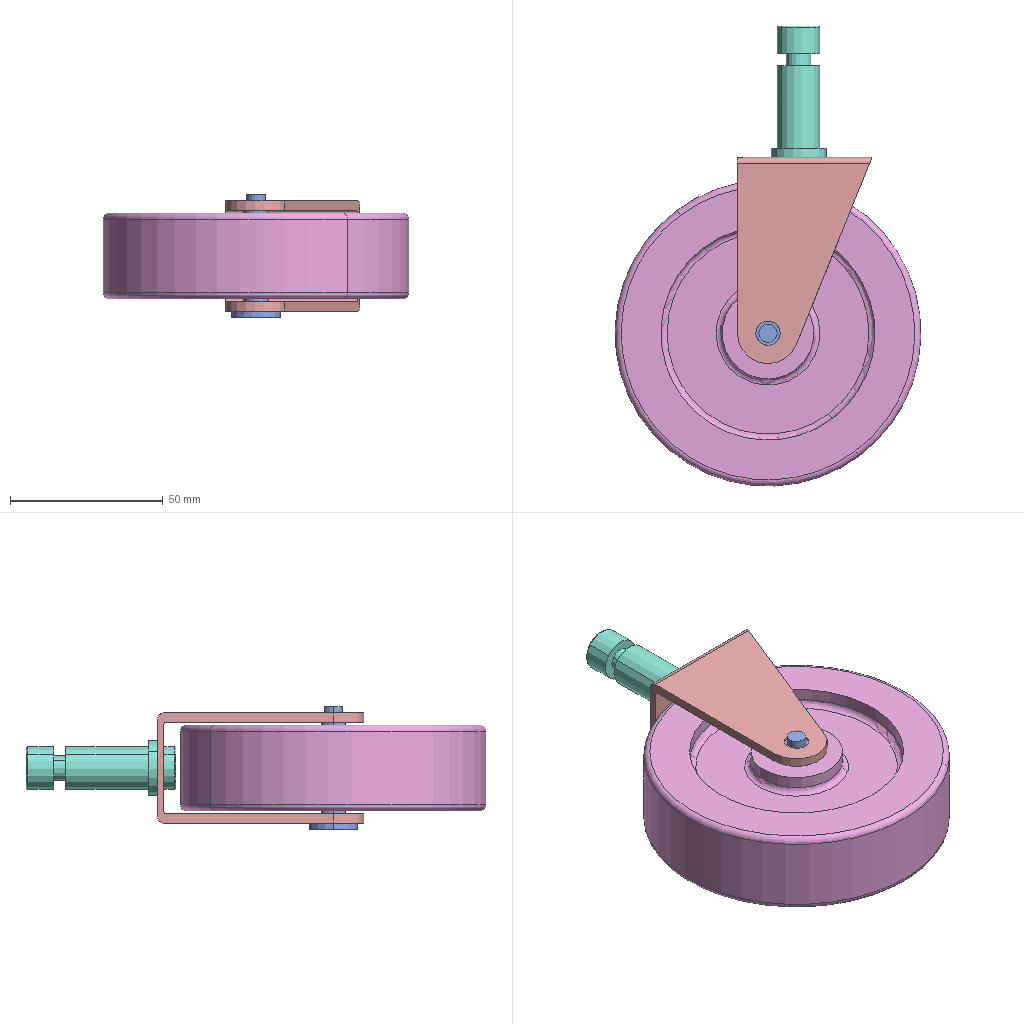Assembly | SolidWorks | 5 different items | 5 placed | box 100 x 150 x 40 mm
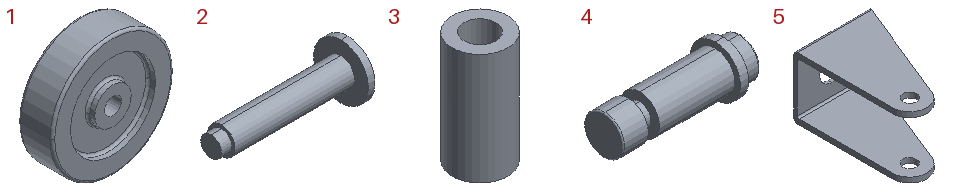Parts list (item | quantity | size | volume | features):
1 | x1 | 100 x 28 x 100 mm | 177907 mm3 | features Fillet 2, Revolution 1
2 | x1 | 40 x 16 x 16 mm | 2246 mm3 | features Revolution 1
3 | x1 | 14 x 14 x 28 mm | 2903 mm3 | features Extrusion 1
4 | x1 | 49 x 18 x 18 mm | 7425 mm3 | features Fillet 1, Revolution 1
5 | x1 | 44 x 67.458 x 36 mm | 14065 mm3 | features ICE 2, Extrusion 1, Fillet 1
Mates (type | each side: item.copy, entity, surface, feature):
Concentric | 2.1 face cylinder Revolve1 | 3.1 face cylinder Boss-Extrude1
Concentric | 5.1 face cylinder Boss-Extrude1 | 1.1 face cylinder Revolve1
Concentric | 5.1 edge | 4.1 face cylinder Revolve1
Coincident | 5.1 face plane Boss-Extrude1 | 4.1 face plane Revolve1
DistanceDim | 1.1 face plane Revolve1 | 5.1 face plane Cut-Extrude1
Coincident | 5.1 face plane Boss-Extrude1 | 2.1 face plane Revolve1
Concentric | 5.1 face cylinder Boss-Extrude1 | 3.1 face cylinder Boss-Extrude1
DistanceDim | 5.1 face plane Cut-Extrude1 | 3.1 face plane Boss-Extrude1